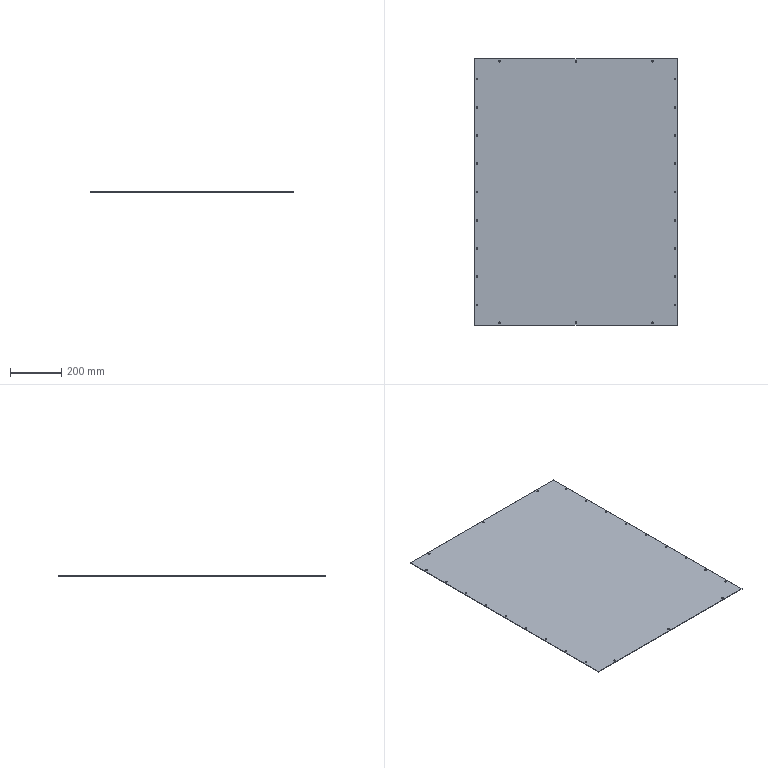Part | SolidWorks | 1 solid | 54 faces | box 794 x 1043 x 2 mm | volume 1654691 mm3 | cylinder 48 | plane 6 | commonest cylinder face diameters 6.5 x48